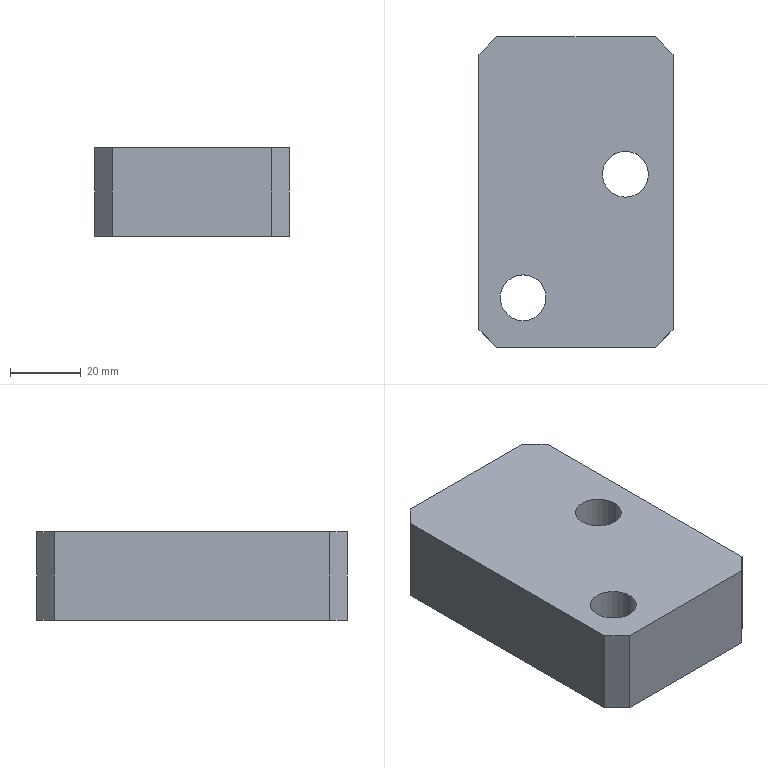Part | STEP file | gslz 2016.10.28-10_id2070_x_t | 1 solid | 16 faces | box 55 x 88 x 25 mm | volume 107688 mm3 | plane 12 | cylinder 4 | commonest cylinder face diameters 13 x2 20 x2
STEP:
#1=CARTESIAN_POINT('',(0.,0.,0.));
#2=DIRECTION('',(0.,0.,1.));
#3=DIRECTION('',(1.,0.,0.));
#4=AXIS2_PLACEMENT_3D('',#1,#2,#3);
#5=CARTESIAN_POINT('',(494.,-313.071,3.));
#6=VERTEX_POINT('',#5);
#7=CARTESIAN_POINT('',(494.,-235.,3.));
#8=VERTEX_POINT('',#7);
#9=CARTESIAN_POINT('',(494.,635.206,3.));
#10=DIRECTION('',(0.,1.,0.));
#11=VECTOR('',#10,1.);
#12=LINE('',#9,#11);
#13=CARTESIAN_POINT('',(494.,627.983,-1.));
#14=DIRECTION('',(-1.,0.,0.));
#15=DIRECTION('',(0.,0.,1.));
#16=AXIS2_PLACEMENT_3D('',#13,#14,#15);
#17=PLANE('',#16);
#18=CARTESIAN_POINT('',(4.,7.223));
#19=DIRECTION('',(0.,1.));
#20=VECTOR('',#19,1.);
#21=LINE('',#18,#20);
#22=(GEOMETRIC_REPRESENTATION_CONTEXT(2)PARAMETRIC_REPRESENTATION_CONTEXT()REPRESENTATION_CONTEXT('',''));
#23=DEFINITIONAL_REPRESENTATION('',(#21),#22);
#24=PCURVE('',#17,#23);
#25=CARTESIAN_POINT('',(-138.966,635.206,3.));
#26=DIRECTION('',(0.,0.,1.));
#27=DIRECTION('',(1.,0.,0.));
#28=AXIS2_PLACEMENT_3D('',#25,#26,#27);
#29=PLANE('',#28);
#30=CARTESIAN_POINT('',(632.966,0.));
#31=DIRECTION('',(0.,1.));
#32=VECTOR('',#31,1.);
#33=LINE('',#30,#32);
#34=(GEOMETRIC_REPRESENTATION_CONTEXT(2)PARAMETRIC_REPRESENTATION_CONTEXT()REPRESENTATION_CONTEXT('',''));
#35=DEFINITIONAL_REPRESENTATION('',(#33),#34);
#36=PCURVE('',#29,#35);
#37=SURFACE_CURVE('',#12,(#24,#36),.PCURVE_S1.);
#38=EDGE_CURVE('',#6,#8,#37,.T.);
#39=ORIENTED_EDGE('',*,*,#38,.T.);
#40=CARTESIAN_POINT('',(494.,-235.,-22.));
#41=VERTEX_POINT('',#40);
#42=CARTESIAN_POINT('',(494.,-235.,-17.));
#43=DIRECTION('',(0.,0.,1.));
#44=VECTOR('',#43,1.);
#45=LINE('',#42,#44);
#46=CARTESIAN_POINT('',(-16.,-862.983));
#47=DIRECTION('',(1.,0.));
#48=VECTOR('',#47,1.);
#49=LINE('',#46,#48);
#50=(GEOMETRIC_REPRESENTATION_CONTEXT(2)PARAMETRIC_REPRESENTATION_CONTEXT()REPRESENTATION_CONTEXT('',''));
#51=DEFINITIONAL_REPRESENTATION('',(#49),#50);
#52=PCURVE('',#17,#51);
#53=CARTESIAN_POINT('',(494.,-235.,-1.));
#54=DIRECTION('',(0.7071,-0.7071,0.));
#55=DIRECTION('',(0.,0.,1.));
#56=AXIS2_PLACEMENT_3D('',#53,#54,#55);
#57=PLANE('',#56);
#58=CARTESIAN_POINT('',(-16.,0.));
#59=DIRECTION('',(1.,0.));
#60=VECTOR('',#59,1.);
#61=LINE('',#58,#60);
#62=(GEOMETRIC_REPRESENTATION_CONTEXT(2)PARAMETRIC_REPRESENTATION_CONTEXT()REPRESENTATION_CONTEXT('',''));
#63=DEFINITIONAL_REPRESENTATION('',(#61),#62);
#64=PCURVE('',#57,#63);
#65=SURFACE_CURVE('',#45,(#52,#64),.PCURVE_S1.);
#66=EDGE_CURVE('',#41,#8,#65,.T.);
#67=ORIENTED_EDGE('',*,*,#66,.F.);
#68=CARTESIAN_POINT('',(494.,-313.071,-22.));
#69=VERTEX_POINT('',#68);
#70=CARTESIAN_POINT('',(494.,635.206,-22.));
#71=DIRECTION('',(0.,1.,0.));
#72=VECTOR('',#71,1.);
#73=LINE('',#70,#72);
#74=CARTESIAN_POINT('',(-21.,7.223));
#75=DIRECTION('',(0.,1.));
#76=VECTOR('',#75,1.);
#77=LINE('',#74,#76);
#78=(GEOMETRIC_REPRESENTATION_CONTEXT(2)PARAMETRIC_REPRESENTATION_CONTEXT()REPRESENTATION_CONTEXT('',''));
#79=DEFINITIONAL_REPRESENTATION('',(#77),#78);
#80=PCURVE('',#17,#79);
#81=CARTESIAN_POINT('',(-138.966,635.206,-22.));
#82=DIRECTION('',(0.,0.,1.));
#83=DIRECTION('',(1.,0.,0.));
#84=AXIS2_PLACEMENT_3D('',#81,#82,#83);
#85=PLANE('',#84);
#86=CARTESIAN_POINT('',(632.966,0.));
#87=DIRECTION('',(0.,1.));
#88=VECTOR('',#87,1.);
#89=LINE('',#86,#88);
#90=(GEOMETRIC_REPRESENTATION_CONTEXT(2)PARAMETRIC_REPRESENTATION_CONTEXT()REPRESENTATION_CONTEXT('',''));
#91=DEFINITIONAL_REPRESENTATION('',(#89),#90);
#92=PCURVE('',#85,#91);
#93=SURFACE_CURVE('',#73,(#80,#92),.PCURVE_S1.);
#94=EDGE_CURVE('',#69,#41,#93,.T.);
#95=ORIENTED_EDGE('',*,*,#94,.F.);
#96=CARTESIAN_POINT('',(494.,-313.071,-1.));
#97=DIRECTION('',(0.,0.,-1.));
#98=VECTOR('',#97,1.);
#99=LINE('',#96,#98);
#100=CARTESIAN_POINT('',(0.,-941.054));
#101=DIRECTION('',(-1.,0.));
#102=VECTOR('',#101,1.);
#103=LINE('',#100,#102);
#104=(GEOMETRIC_REPRESENTATION_CONTEXT(2)PARAMETRIC_REPRESENTATION_CONTEXT()REPRESENTATION_CONTEXT('',''));
#105=DEFINITIONAL_REPRESENTATION('',(#103),#104);
#106=PCURVE('',#17,#105);
#107=CARTESIAN_POINT('',(497.464,-316.536,49.));
#108=DIRECTION('',(0.7071,0.7071,0.));
#109=DIRECTION('',(0.,0.,1.));
#110=AXIS2_PLACEMENT_3D('',#107,#108,#109);
#111=PLANE('',#110);
#112=CARTESIAN_POINT('',(-50.,-4.899));
#113=DIRECTION('',(-1.,0.));
#114=VECTOR('',#113,1.);
#115=LINE('',#112,#114);
#116=(GEOMETRIC_REPRESENTATION_CONTEXT(2)PARAMETRIC_REPRESENTATION_CONTEXT()REPRESENTATION_CONTEXT('',''));
#117=DEFINITIONAL_REPRESENTATION('',(#115),#116);
#118=PCURVE('',#111,#117);
#119=SURFACE_CURVE('',#99,(#106,#118),.PCURVE_S1.);
#120=EDGE_CURVE('',#6,#69,#119,.T.);
#121=ORIENTED_EDGE('',*,*,#120,.F.);
#122=EDGE_LOOP('',(#39,#67,#95,#121));
#123=FACE_BOUND('',#122,.T.);
#124=ADVANCED_FACE('',(#123),#17,.T.);
#125=CARTESIAN_POINT('',(549.,-235.,-22.));
#126=VERTEX_POINT('',#125);
#127=CARTESIAN_POINT('',(549.,-313.071,-22.));
#128=VERTEX_POINT('',#127);
#129=CARTESIAN_POINT('',(549.,635.206,-22.));
#130=DIRECTION('',(0.,-1.,0.));
#131=VECTOR('',#130,1.);
#132=LINE('',#129,#131);
#133=CARTESIAN_POINT('',(549.,627.983,-1.));
#134=DIRECTION('',(1.,0.,0.));
#135=DIRECTION('',(0.,0.,-1.));
#136=AXIS2_PLACEMENT_3D('',#133,#134,#135);
#137=PLANE('',#136);
#138=CARTESIAN_POINT('',(21.,7.223));
#139=DIRECTION('',(0.,-1.));
#140=VECTOR('',#139,1.);
#141=LINE('',#138,#140);
#142=(GEOMETRIC_REPRESENTATION_CONTEXT(2)PARAMETRIC_REPRESENTATION_CONTEXT()REPRESENTATION_CONTEXT('',''));
#143=DEFINITIONAL_REPRESENTATION('',(#141),#142);
#144=PCURVE('',#137,#143);
#145=CARTESIAN_POINT('',(687.966,0.));
#146=DIRECTION('',(0.,-1.));
#147=VECTOR('',#146,1.);
#148=LINE('',#145,#147);
#149=(GEOMETRIC_REPRESENTATION_CONTEXT(2)PARAMETRIC_REPRESENTATION_CONTEXT()REPRESENTATION_CONTEXT('',''));
#150=DEFINITIONAL_REPRESENTATION('',(#148),#149);
#151=PCURVE('',#85,#150);
#152=SURFACE_CURVE('',#132,(#144,#151),.PCURVE_S1.);
#153=EDGE_CURVE('',#126,#128,#152,.T.);
#154=ORIENTED_EDGE('',*,*,#153,.F.);
#155=CARTESIAN_POINT('',(549.,-235.,3.));
#156=VERTEX_POINT('',#155);
#157=CARTESIAN_POINT('',(549.,-235.,3.));
#158=DIRECTION('',(0.,0.,-1.));
#159=VECTOR('',#158,1.);
#160=LINE('',#157,#159);
#161=CARTESIAN_POINT('',(-4.,-862.983));
#162=DIRECTION('',(1.,0.));
#163=VECTOR('',#162,1.);
#164=LINE('',#161,#163);
#165=(GEOMETRIC_REPRESENTATION_CONTEXT(2)PARAMETRIC_REPRESENTATION_CONTEXT()REPRESENTATION_CONTEXT('',''));
#166=DEFINITIONAL_REPRESENTATION('',(#164),#165);
#167=PCURVE('',#137,#166);
#168=CARTESIAN_POINT('',(544.,-230.,4.));
#169=DIRECTION('',(-0.7071,-0.7071,0.));
#170=DIRECTION('',(0.,0.,1.));
#171=AXIS2_PLACEMENT_3D('',#168,#169,#170);
#172=PLANE('',#171);
#173=CARTESIAN_POINT('',(-1.,-7.071));
#174=DIRECTION('',(-1.,0.));
#175=VECTOR('',#174,1.);
#176=LINE('',#173,#175);
#177=(GEOMETRIC_REPRESENTATION_CONTEXT(2)PARAMETRIC_REPRESENTATION_CONTEXT()REPRESENTATION_CONTEXT('',''));
#178=DEFINITIONAL_REPRESENTATION('',(#176),#177);
#179=PCURVE('',#172,#178);
#180=SURFACE_CURVE('',#160,(#167,#179),.PCURVE_S1.);
#181=EDGE_CURVE('',#156,#126,#180,.T.);
#182=ORIENTED_EDGE('',*,*,#181,.F.);
#183=CARTESIAN_POINT('',(549.,-313.071,3.));
#184=VERTEX_POINT('',#183);
#185=CARTESIAN_POINT('',(549.,635.206,3.));
#186=DIRECTION('',(0.,-1.,0.));
#187=VECTOR('',#186,1.);
#188=LINE('',#185,#187);
#189=CARTESIAN_POINT('',(-4.,7.223));
#190=DIRECTION('',(0.,-1.));
#191=VECTOR('',#190,1.);
#192=LINE('',#189,#191);
#193=(GEOMETRIC_REPRESENTATION_CONTEXT(2)PARAMETRIC_REPRESENTATION_CONTEXT()REPRESENTATION_CONTEXT('',''));
#194=DEFINITIONAL_REPRESENTATION('',(#192),#193);
#195=PCURVE('',#137,#194);
#196=CARTESIAN_POINT('',(687.966,0.));
#197=DIRECTION('',(0.,-1.));
#198=VECTOR('',#197,1.);
#199=LINE('',#196,#198);
#200=(GEOMETRIC_REPRESENTATION_CONTEXT(2)PARAMETRIC_REPRESENTATION_CONTEXT()REPRESENTATION_CONTEXT('',''));
#201=DEFINITIONAL_REPRESENTATION('',(#199),#200);
#202=PCURVE('',#29,#201);
#203=SURFACE_CURVE('',#188,(#195,#202),.PCURVE_S1.);
#204=EDGE_CURVE('',#156,#184,#203,.T.);
#205=ORIENTED_EDGE('',*,*,#204,.T.);
#206=CARTESIAN_POINT('',(549.,-313.071,-1.));
#207=DIRECTION('',(0.,0.,1.));
#208=VECTOR('',#207,1.);
#209=LINE('',#206,#208);
#210=CARTESIAN_POINT('',(0.,-941.054));
#211=DIRECTION('',(-1.,0.));
#212=VECTOR('',#211,1.);
#213=LINE('',#210,#212);
#214=(GEOMETRIC_REPRESENTATION_CONTEXT(2)PARAMETRIC_REPRESENTATION_CONTEXT()REPRESENTATION_CONTEXT('',''));
#215=DEFINITIONAL_REPRESENTATION('',(#213),#214);
#216=PCURVE('',#137,#215);
#217=CARTESIAN_POINT('',(547.536,-314.536,-1.));
#218=DIRECTION('',(-0.7071,0.7071,0.));
#219=DIRECTION('',(0.,0.,1.));
#220=AXIS2_PLACEMENT_3D('',#217,#218,#219);
#221=PLANE('',#220);
#222=CARTESIAN_POINT('',(0.,2.071));
#223=DIRECTION('',(1.,0.));
#224=VECTOR('',#223,1.);
#225=LINE('',#222,#224);
#226=(GEOMETRIC_REPRESENTATION_CONTEXT(2)PARAMETRIC_REPRESENTATION_CONTEXT()REPRESENTATION_CONTEXT('',''));
#227=DEFINITIONAL_REPRESENTATION('',(#225),#226);
#228=PCURVE('',#221,#227);
#229=SURFACE_CURVE('',#209,(#216,#228),.PCURVE_S1.);
#230=EDGE_CURVE('',#128,#184,#229,.T.);
#231=ORIENTED_EDGE('',*,*,#230,.F.);
#232=EDGE_LOOP('',(#154,#182,#205,#231));
#233=FACE_BOUND('',#232,.T.);
#234=ADVANCED_FACE('',(#233),#137,.T.);
#235=CARTESIAN_POINT('',(506.5,-314.,-22.));
#236=VERTEX_POINT('',#235);
#237=CARTESIAN_POINT('',(506.5,-294.,-22.));
#238=VERTEX_POINT('',#237);
#239=CARTESIAN_POINT('',(506.5,-304.,-22.));
#240=DIRECTION('',(0.,0.,-1.));
#241=DIRECTION('',(0.,-1.,0.));
#242=AXIS2_PLACEMENT_3D('',#239,#240,#241);
#243=CIRCLE('',#242,10.);
#244=CARTESIAN_POINT('',(645.466,-949.206));
#245=CARTESIAN_POINT('',(628.146,-949.206));
#246=CARTESIAN_POINT('',(636.806,-934.206));
#247=CARTESIAN_POINT('',(645.466,-919.206));
#248=CARTESIAN_POINT('',(654.127,-934.206));
#249=CARTESIAN_POINT('',(662.787,-949.206));
#250=CARTESIAN_POINT('',(645.466,-949.206));
#251=(BOUNDED_CURVE()B_SPLINE_CURVE(2,(#244,#245,#246,#247,#248,#249,#250),.UNSPECIFIED.,.T.,.F.)B_SPLINE_CURVE_WITH_KNOTS((1,2,2,2,2,1),(-2.094,0.,2.094,4.189,6.283,8.378),.UNSPECIFIED.)CURVE()GEOMETRIC_REPRESENTATION_ITEM()RATIONAL_B_SPLINE_CURVE((1.,0.5,1.,0.5,1.,0.5,1.))REPRESENTATION_ITEM(''));
#252=(GEOMETRIC_REPRESENTATION_CONTEXT(2)PARAMETRIC_REPRESENTATION_CONTEXT()REPRESENTATION_CONTEXT('',''));
#253=DEFINITIONAL_REPRESENTATION('',(#251),#252);
#254=PCURVE('',#85,#253);
#255=CARTESIAN_POINT('',(506.5,-304.,3.));
#256=DIRECTION('',(0.,0.,1.));
#257=DIRECTION('',(1.,0.,0.));
#258=AXIS2_PLACEMENT_3D('',#255,#256,#257);
#259=CYLINDRICAL_SURFACE('',#258,10.);
#260=CARTESIAN_POINT('',(4.712,-25.));
#261=DIRECTION('',(-1.,0.));
#262=VECTOR('',#261,1.);
#263=LINE('',#260,#262);
#264=(GEOMETRIC_REPRESENTATION_CONTEXT(2)PARAMETRIC_REPRESENTATION_CONTEXT()REPRESENTATION_CONTEXT('',''));
#265=DEFINITIONAL_REPRESENTATION('',(#263),#264);
#266=PCURVE('',#259,#265);
#267=SURFACE_CURVE('',#243,(#254,#266),.PCURVE_S1.);
#268=EDGE_CURVE('',#236,#238,#267,.T.);
#269=ORIENTED_EDGE('',*,*,#268,.F.);
#270=CARTESIAN_POINT('',(506.5,-304.,-22.));
#271=DIRECTION('',(0.,0.,-1.));
#272=DIRECTION('',(0.,-1.,0.));
#273=AXIS2_PLACEMENT_3D('',#270,#271,#272);
#274=CIRCLE('',#273,10.);
#275=CARTESIAN_POINT('',(645.466,-949.206));
#276=CARTESIAN_POINT('',(628.146,-949.206));
#277=CARTESIAN_POINT('',(636.806,-934.206));
#278=CARTESIAN_POINT('',(645.466,-919.206));
#279=CARTESIAN_POINT('',(654.127,-934.206));
#280=CARTESIAN_POINT('',(662.787,-949.206));
#281=CARTESIAN_POINT('',(645.466,-949.206));
#282=(BOUNDED_CURVE()B_SPLINE_CURVE(2,(#275,#276,#277,#278,#279,#280,#281),.UNSPECIFIED.,.T.,.F.)B_SPLINE_CURVE_WITH_KNOTS((1,2,2,2,2,1),(-2.094,0.,2.094,4.189,6.283,8.378),.UNSPECIFIED.)CURVE()GEOMETRIC_REPRESENTATION_ITEM()RATIONAL_B_SPLINE_CURVE((1.,0.5,1.,0.5,1.,0.5,1.))REPRESENTATION_ITEM(''));
#283=(GEOMETRIC_REPRESENTATION_CONTEXT(2)PARAMETRIC_REPRESENTATION_CONTEXT()REPRESENTATION_CONTEXT('',''));
#284=DEFINITIONAL_REPRESENTATION('',(#282),#283);
#285=PCURVE('',#85,#284);
#286=CARTESIAN_POINT('',(10.996,-25.));
#287=DIRECTION('',(-1.,0.));
#288=VECTOR('',#287,1.);
#289=LINE('',#286,#288);
#290=(GEOMETRIC_REPRESENTATION_CONTEXT(2)PARAMETRIC_REPRESENTATION_CONTEXT()REPRESENTATION_CONTEXT('',''));
#291=DEFINITIONAL_REPRESENTATION('',(#289),#290);
#292=PCURVE('',#259,#291);
#293=SURFACE_CURVE('',#274,(#285,#292),.PCURVE_S1.);
#294=EDGE_CURVE('',#238,#236,#293,.T.);
#295=ORIENTED_EDGE('',*,*,#294,.F.);
#296=EDGE_LOOP('',(#269,#295));
#297=FACE_BOUND('',#296,.T.);
#298=CARTESIAN_POINT('',(535.5,-279.,-22.));
#299=VERTEX_POINT('',#298);
#300=CARTESIAN_POINT('',(535.5,-259.,-22.));
#301=VERTEX_POINT('',#300);
#302=CARTESIAN_POINT('',(535.5,-269.,-22.));
#303=DIRECTION('',(0.,0.,1.));
#304=DIRECTION('',(0.,-1.,0.));
#305=AXIS2_PLACEMENT_3D('',#302,#303,#304);
#306=CIRCLE('',#305,10.);
#307=CARTESIAN_POINT('',(674.466,-904.206));
#308=DIRECTION('',(0.,-1.));
#309=AXIS2_PLACEMENT_2D('',#307,#308);
#310=CIRCLE('',#309,10.);
#311=(GEOMETRIC_REPRESENTATION_CONTEXT(2)PARAMETRIC_REPRESENTATION_CONTEXT()REPRESENTATION_CONTEXT('',''));
#312=DEFINITIONAL_REPRESENTATION('',(#310),#311);
#313=PCURVE('',#85,#312);
#314=CARTESIAN_POINT('',(535.5,-269.,3.));
#315=DIRECTION('',(0.,0.,1.));
#316=DIRECTION('',(1.,0.,0.));
#317=AXIS2_PLACEMENT_3D('',#314,#315,#316);
#318=CYLINDRICAL_SURFACE('',#317,10.);
#319=CARTESIAN_POINT('',(4.712,-25.));
#320=DIRECTION('',(1.,0.));
#321=VECTOR('',#320,1.);
#322=LINE('',#319,#321);
#323=(GEOMETRIC_REPRESENTATION_CONTEXT(2)PARAMETRIC_REPRESENTATION_CONTEXT()REPRESENTATION_CONTEXT('',''));
#324=DEFINITIONAL_REPRESENTATION('',(#322),#323);
#325=PCURVE('',#318,#324);
#326=SURFACE_CURVE('',#306,(#313,#325),.PCURVE_S1.);
#327=EDGE_CURVE('',#299,#301,#326,.T.);
#328=ORIENTED_EDGE('',*,*,#327,.T.);
#329=CARTESIAN_POINT('',(535.5,-269.,-22.));
#330=DIRECTION('',(0.,0.,1.));
#331=DIRECTION('',(0.,-1.,0.));
#332=AXIS2_PLACEMENT_3D('',#329,#330,#331);
#333=CIRCLE('',#332,10.);
#334=CARTESIAN_POINT('',(674.466,-904.206));
#335=DIRECTION('',(0.,-1.));
#336=AXIS2_PLACEMENT_2D('',#334,#335);
#337=CIRCLE('',#336,10.);
#338=(GEOMETRIC_REPRESENTATION_CONTEXT(2)PARAMETRIC_REPRESENTATION_CONTEXT()REPRESENTATION_CONTEXT('',''));
#339=DEFINITIONAL_REPRESENTATION('',(#337),#338);
#340=PCURVE('',#85,#339);
#341=CARTESIAN_POINT('',(-1.571,-25.));
#342=DIRECTION('',(1.,0.));
#343=VECTOR('',#342,1.);
#344=LINE('',#341,#343);
#345=(GEOMETRIC_REPRESENTATION_CONTEXT(2)PARAMETRIC_REPRESENTATION_CONTEXT()REPRESENTATION_CONTEXT('',''));
#346=DEFINITIONAL_REPRESENTATION('',(#344),#345);
#347=PCURVE('',#318,#346);
#348=SURFACE_CURVE('',#333,(#340,#347),.PCURVE_S1.);
#349=EDGE_CURVE('',#301,#299,#348,.T.);
#350=ORIENTED_EDGE('',*,*,#349,.T.);
#351=EDGE_LOOP('',(#328,#350));
#352=FACE_BOUND('',#351,.T.);
#353=CARTESIAN_POINT('',(499.,-230.,-22.));
#354=VERTEX_POINT('',#353);
#355=CARTESIAN_POINT('',(544.,-230.,-22.));
#356=VERTEX_POINT('',#355);
#357=CARTESIAN_POINT('',(-138.966,-230.,-22.));
#358=DIRECTION('',(1.,0.,0.));
#359=VECTOR('',#358,1.);
#360=LINE('',#357,#359);
#361=CARTESIAN_POINT('',(0.,-865.206));
#362=DIRECTION('',(1.,0.));
#363=VECTOR('',#362,1.);
#364=LINE('',#361,#363);
#365=(GEOMETRIC_REPRESENTATION_CONTEXT(2)PARAMETRIC_REPRESENTATION_CONTEXT()REPRESENTATION_CONTEXT('',''));
#366=DEFINITIONAL_REPRESENTATION('',(#364),#365);
#367=PCURVE('',#85,#366);
#368=CARTESIAN_POINT('',(-137.035,-230.,4.));
#369=DIRECTION('',(0.,1.,0.));
#370=DIRECTION('',(-1.,0.,0.));
#371=AXIS2_PLACEMENT_3D('',#368,#369,#370);
#372=PLANE('',#371);
#373=CARTESIAN_POINT('',(1.931,-26.));
#374=DIRECTION('',(-1.,0.));
#375=VECTOR('',#374,1.);
#376=LINE('',#373,#375);
#377=(GEOMETRIC_REPRESENTATION_CONTEXT(2)PARAMETRIC_REPRESENTATION_CONTEXT()REPRESENTATION_CONTEXT('',''));
#378=DEFINITIONAL_REPRESENTATION('',(#376),#377);
#379=PCURVE('',#372,#378);
#380=SURFACE_CURVE('',#360,(#367,#379),.PCURVE_S1.);
#381=EDGE_CURVE('',#354,#356,#380,.T.);
#382=ORIENTED_EDGE('',*,*,#381,.T.);
#383=CARTESIAN_POINT('',(544.,-230.,-22.));
#384=DIRECTION('',(-0.7071,0.7071,0.));
#385=VECTOR('',#384,1.);
#386=LINE('',#383,#385);
#387=CARTESIAN_POINT('',(682.966,-865.206));
#388=DIRECTION('',(-0.7071,0.7071));
#389=VECTOR('',#388,1.);
#390=LINE('',#387,#389);
#391=(GEOMETRIC_REPRESENTATION_CONTEXT(2)PARAMETRIC_REPRESENTATION_CONTEXT()REPRESENTATION_CONTEXT('',''));
#392=DEFINITIONAL_REPRESENTATION('',(#390),#391);
#393=PCURVE('',#85,#392);
#394=CARTESIAN_POINT('',(-26.,0.));
#395=DIRECTION('',(0.,1.));
#396=VECTOR('',#395,1.);
#397=LINE('',#394,#396);
#398=(GEOMETRIC_REPRESENTATION_CONTEXT(2)PARAMETRIC_REPRESENTATION_CONTEXT()REPRESENTATION_CONTEXT('',''));
#399=DEFINITIONAL_REPRESENTATION('',(#397),#398);
#400=PCURVE('',#172,#399);
#401=SURFACE_CURVE('',#386,(#393,#400),.PCURVE_S1.);
#402=EDGE_CURVE('',#126,#356,#401,.T.);
#403=ORIENTED_EDGE('',*,*,#402,.F.);
#404=ORIENTED_EDGE('',*,*,#153,.T.);
#405=CARTESIAN_POINT('',(544.071,-318.,-22.));
#406=VERTEX_POINT('',#405);
#407=CARTESIAN_POINT('',(547.536,-314.536,-22.));
#408=DIRECTION('',(0.7071,0.7071,0.));
#409=VECTOR('',#408,1.);
#410=LINE('',#407,#409);
#411=CARTESIAN_POINT('',(686.502,-949.741));
#412=DIRECTION('',(0.7071,0.7071));
#413=VECTOR('',#412,1.);
#414=LINE('',#411,#413);
#415=(GEOMETRIC_REPRESENTATION_CONTEXT(2)PARAMETRIC_REPRESENTATION_CONTEXT()REPRESENTATION_CONTEXT('',''));
#416=DEFINITIONAL_REPRESENTATION('',(#414),#415);
#417=PCURVE('',#85,#416);
#418=CARTESIAN_POINT('',(-21.,0.));
#419=DIRECTION('',(0.,1.));
#420=VECTOR('',#419,1.);
#421=LINE('',#418,#420);
#422=(GEOMETRIC_REPRESENTATION_CONTEXT(2)PARAMETRIC_REPRESENTATION_CONTEXT()REPRESENTATION_CONTEXT('',''));
#423=DEFINITIONAL_REPRESENTATION('',(#421),#422);
#424=PCURVE('',#221,#423);
#425=SURFACE_CURVE('',#410,(#417,#424),.PCURVE_S1.);
#426=EDGE_CURVE('',#406,#128,#425,.T.);
#427=ORIENTED_EDGE('',*,*,#426,.F.);
#428=CARTESIAN_POINT('',(498.929,-318.,-22.));
#429=VERTEX_POINT('',#428);
#430=CARTESIAN_POINT('',(-138.966,-318.,-22.));
#431=DIRECTION('',(-1.,0.,0.));
#432=VECTOR('',#431,1.);
#433=LINE('',#430,#432);
#434=CARTESIAN_POINT('',(0.,-953.206));
#435=DIRECTION('',(-1.,0.));
#436=VECTOR('',#435,1.);
#437=LINE('',#434,#436);
#438=(GEOMETRIC_REPRESENTATION_CONTEXT(2)PARAMETRIC_REPRESENTATION_CONTEXT()REPRESENTATION_CONTEXT('',''));
#439=DEFINITIONAL_REPRESENTATION('',(#437),#438);
#440=PCURVE('',#85,#439);
#441=CARTESIAN_POINT('',(501.5,-318.,49.));
#442=DIRECTION('',(0.,-1.,0.));
#443=DIRECTION('',(0.,0.,1.));
#444=AXIS2_PLACEMENT_3D('',#441,#442,#443);
#445=PLANE('',#444);
#446=CARTESIAN_POINT('',(-71.,640.466));
#447=DIRECTION('',(0.,1.));
#448=VECTOR('',#447,1.);
#449=LINE('',#446,#448);
#450=(GEOMETRIC_REPRESENTATION_CONTEXT(2)PARAMETRIC_REPRESENTATION_CONTEXT()REPRESENTATION_CONTEXT('',''));
#451=DEFINITIONAL_REPRESENTATION('',(#449),#450);
#452=PCURVE('',#445,#451);
#453=SURFACE_CURVE('',#433,(#440,#452),.PCURVE_S1.);
#454=EDGE_CURVE('',#406,#429,#453,.T.);
#455=ORIENTED_EDGE('',*,*,#454,.T.);
#456=CARTESIAN_POINT('',(497.464,-316.536,-22.));
#457=DIRECTION('',(0.7071,-0.7071,0.));
#458=VECTOR('',#457,1.);
#459=LINE('',#456,#458);
#460=CARTESIAN_POINT('',(636.431,-951.741));
#461=DIRECTION('',(0.7071,-0.7071));
#462=VECTOR('',#461,1.);
#463=LINE('',#460,#462);
#464=(GEOMETRIC_REPRESENTATION_CONTEXT(2)PARAMETRIC_REPRESENTATION_CONTEXT()REPRESENTATION_CONTEXT('',''));
#465=DEFINITIONAL_REPRESENTATION('',(#463),#464);
#466=PCURVE('',#85,#465);
#467=CARTESIAN_POINT('',(-71.,0.));
#468=DIRECTION('',(0.,1.));
#469=VECTOR('',#468,1.);
#470=LINE('',#467,#469);
#471=(GEOMETRIC_REPRESENTATION_CONTEXT(2)PARAMETRIC_REPRESENTATION_CONTEXT()REPRESENTATION_CONTEXT('',''));
#472=DEFINITIONAL_REPRESENTATION('',(#470),#471);
#473=PCURVE('',#111,#472);
#474=SURFACE_CURVE('',#459,(#466,#473),.PCURVE_S1.);
#475=EDGE_CURVE('',#69,#429,#474,.T.);
#476=ORIENTED_EDGE('',*,*,#475,.F.);
#477=ORIENTED_EDGE('',*,*,#94,.T.);
#478=CARTESIAN_POINT('',(494.,-235.,-22.));
#479=DIRECTION('',(-0.7071,-0.7071,0.));
#480=VECTOR('',#479,1.);
#481=LINE('',#478,#480);
#482=CARTESIAN_POINT('',(632.966,-870.206));
#483=DIRECTION('',(-0.7071,-0.7071));
#484=VECTOR('',#483,1.);
#485=LINE('',#482,#484);
#486=(GEOMETRIC_REPRESENTATION_CONTEXT(2)PARAMETRIC_REPRESENTATION_CONTEXT()REPRESENTATION_CONTEXT('',''));
#487=DEFINITIONAL_REPRESENTATION('',(#485),#486);
#488=PCURVE('',#85,#487);
#489=CARTESIAN_POINT('',(-21.,0.));
#490=DIRECTION('',(0.,1.));
#491=VECTOR('',#490,1.);
#492=LINE('',#489,#491);
#493=(GEOMETRIC_REPRESENTATION_CONTEXT(2)PARAMETRIC_REPRESENTATION_CONTEXT()REPRESENTATION_CONTEXT('',''));
#494=DEFINITIONAL_REPRESENTATION('',(#492),#493);
#495=PCURVE('',#57,#494);
#496=SURFACE_CURVE('',#481,(#488,#495),.PCURVE_S1.);
#497=EDGE_CURVE('',#354,#41,#496,.T.);
#498=ORIENTED_EDGE('',*,*,#497,.F.);
#499=EDGE_LOOP('',(#382,#403,#404,#427,#455,#476,#477,#498));
#500=FACE_BOUND('',#499,.T.);
#501=ADVANCED_FACE('',(#297,#352,#500),#85,.F.);
#502=CARTESIAN_POINT('',(535.5,-275.5,3.));
#503=VERTEX_POINT('',#502);
#504=CARTESIAN_POINT('',(535.5,-269.,3.));
#505=DIRECTION('',(0.,0.,-1.));
#506=DIRECTION('',(0.,-1.,0.));
#507=AXIS2_PLACEMENT_3D('',#504,#505,#506);
#508=CIRCLE('',#507,6.5);
#509=CARTESIAN_POINT('',(674.466,-910.706));
#510=CARTESIAN_POINT('',(663.208,-910.706));
#511=CARTESIAN_POINT('',(668.837,-900.956));
#512=CARTESIAN_POINT('',(674.466,-891.206));
#513=CARTESIAN_POINT('',(680.096,-900.956));
#514=CARTESIAN_POINT('',(685.725,-910.706));
#515=CARTESIAN_POINT('',(674.466,-910.706));
#516=(BOUNDED_CURVE()B_SPLINE_CURVE(2,(#509,#510,#511,#512,#513,#514,#515),.UNSPECIFIED.,.T.,.F.)B_SPLINE_CURVE_WITH_KNOTS((1,2,2,2,2,1),(-2.094,0.,2.094,4.189,6.283,8.378),.UNSPECIFIED.)CURVE()GEOMETRIC_REPRESENTATION_ITEM()RATIONAL_B_SPLINE_CURVE((1.,0.5,1.,0.5,1.,0.5,1.))REPRESENTATION_ITEM(''));
#517=(GEOMETRIC_REPRESENTATION_CONTEXT(2)PARAMETRIC_REPRESENTATION_CONTEXT()REPRESENTATION_CONTEXT('',''));
#518=DEFINITIONAL_REPRESENTATION('',(#516),#517);
#519=PCURVE('',#29,#518);
#520=CARTESIAN_POINT('',(535.5,-269.,-84.));
#521=DIRECTION('',(0.,0.,1.));
#522=DIRECTION('',(0.,-1.,0.));
#523=AXIS2_PLACEMENT_3D('',#520,#521,#522);
#524=CYLINDRICAL_SURFACE('',#523,6.5);
#525=CARTESIAN_POINT('',(6.283,87.));
#526=DIRECTION('',(-1.,0.));
#527=VECTOR('',#526,1.);
#528=LINE('',#525,#527);
#529=(GEOMETRIC_REPRESENTATION_CONTEXT(2)PARAMETRIC_REPRESENTATION_CONTEXT()REPRESENTATION_CONTEXT('',''));
#530=DEFINITIONAL_REPRESENTATION('',(#528),#529);
#531=PCURVE('',#524,#530);
#532=SURFACE_CURVE('',#508,(#519,#531),.PCURVE_S1.);
#533=EDGE_CURVE('',#503,#503,#532,.T.);
#534=ORIENTED_EDGE('',*,*,#533,.T.);
#535=EDGE_LOOP('',(#534));
#536=FACE_BOUND('',#535,.T.);
#537=CARTESIAN_POINT('',(506.5,-310.5,3.));
#538=VERTEX_POINT('',#537);
#539=CARTESIAN_POINT('',(506.5,-304.,3.));
#540=DIRECTION('',(0.,0.,-1.));
#541=DIRECTION('',(0.,-1.,0.));
#542=AXIS2_PLACEMENT_3D('',#539,#540,#541);
#543=CIRCLE('',#542,6.5);
#544=CARTESIAN_POINT('',(645.466,-945.706));
#545=CARTESIAN_POINT('',(634.208,-945.706));
#546=CARTESIAN_POINT('',(639.837,-935.956));
#547=CARTESIAN_POINT('',(645.466,-926.206));
#548=CARTESIAN_POINT('',(651.096,-935.956));
#549=CARTESIAN_POINT('',(656.725,-945.706));
#550=CARTESIAN_POINT('',(645.466,-945.706));
#551=(BOUNDED_CURVE()B_SPLINE_CURVE(2,(#544,#545,#546,#547,#548,#549,#550),.UNSPECIFIED.,.T.,.F.)B_SPLINE_CURVE_WITH_KNOTS((1,2,2,2,2,1),(-2.094,0.,2.094,4.189,6.283,8.378),.UNSPECIFIED.)CURVE()GEOMETRIC_REPRESENTATION_ITEM()RATIONAL_B_SPLINE_CURVE((1.,0.5,1.,0.5,1.,0.5,1.))REPRESENTATION_ITEM(''));
#552=(GEOMETRIC_REPRESENTATION_CONTEXT(2)PARAMETRIC_REPRESENTATION_CONTEXT()REPRESENTATION_CONTEXT('',''));
#553=DEFINITIONAL_REPRESENTATION('',(#551),#552);
#554=PCURVE('',#29,#553);
#555=CARTESIAN_POINT('',(506.5,-304.,-84.));
#556=DIRECTION('',(0.,0.,1.));
#557=DIRECTION('',(0.,-1.,0.));
#558=AXIS2_PLACEMENT_3D('',#555,#556,#557);
#559=CYLINDRICAL_SURFACE('',#558,6.5);
#560=CARTESIAN_POINT('',(6.283,87.));
#561=DIRECTION('',(-1.,0.));
#562=VECTOR('',#561,1.);
#563=LINE('',#560,#562);
#564=(GEOMETRIC_REPRESENTATION_CONTEXT(2)PARAMETRIC_REPRESENTATION_CONTEXT()REPRESENTATION_CONTEXT('',''));
#565=DEFINITIONAL_REPRESENTATION('',(#563),#564);
#566=PCURVE('',#559,#565);
#567=SURFACE_CURVE('',#543,(#554,#566),.PCURVE_S1.);
#568=EDGE_CURVE('',#538,#538,#567,.T.);
#569=ORIENTED_EDGE('',*,*,#568,.T.);
#570=EDGE_LOOP('',(#569));
#571=FACE_BOUND('',#570,.T.);
#572=ORIENTED_EDGE('',*,*,#204,.F.);
#573=CARTESIAN_POINT('',(544.,-230.,3.));
#574=VERTEX_POINT('',#573);
#575=CARTESIAN_POINT('',(-227.586,541.586,3.));
#576=DIRECTION('',(0.7071,-0.7071,0.));
#577=VECTOR('',#576,1.);
#578=LINE('',#575,#577);
#579=CARTESIAN_POINT('',(-88.62,-93.62));
#580=DIRECTION('',(0.7071,-0.7071));
#581=VECTOR('',#580,1.);
#582=LINE('',#579,#581);
#583=(GEOMETRIC_REPRESENTATION_CONTEXT(2)PARAMETRIC_REPRESENTATION_CONTEXT()REPRESENTATION_CONTEXT('',''));
#584=DEFINITIONAL_REPRESENTATION('',(#582),#583);
#585=PCURVE('',#29,#584);
#586=CARTESIAN_POINT('',(-1.,1091.187));
#587=DIRECTION('',(0.,-1.));
#588=VECTOR('',#587,1.);
#589=LINE('',#586,#588);
#590=(GEOMETRIC_REPRESENTATION_CONTEXT(2)PARAMETRIC_REPRESENTATION_CONTEXT()REPRESENTATION_CONTEXT('',''));
#591=DEFINITIONAL_REPRESENTATION('',(#589),#590);
#592=PCURVE('',#172,#591);
#593=SURFACE_CURVE('',#578,(#585,#592),.PCURVE_S1.);
#594=EDGE_CURVE('',#574,#156,#593,.T.);
#595=ORIENTED_EDGE('',*,*,#594,.F.);
#596=CARTESIAN_POINT('',(499.,-230.,3.));
#597=VERTEX_POINT('',#596);
#598=CARTESIAN_POINT('',(-138.966,-230.,3.));
#599=DIRECTION('',(1.,0.,0.));
#600=VECTOR('',#599,1.);
#601=LINE('',#598,#600);
#602=CARTESIAN_POINT('',(0.,-865.206));
#603=DIRECTION('',(1.,0.));
#604=VECTOR('',#603,1.);
#605=LINE('',#602,#604);
#606=(GEOMETRIC_REPRESENTATION_CONTEXT(2)PARAMETRIC_REPRESENTATION_CONTEXT()REPRESENTATION_CONTEXT('',''));
#607=DEFINITIONAL_REPRESENTATION('',(#605),#606);
#608=PCURVE('',#29,#607);
#609=CARTESIAN_POINT('',(1.931,-1.));
#610=DIRECTION('',(-1.,0.));
#611=VECTOR('',#610,1.);
#612=LINE('',#609,#611);
#613=(GEOMETRIC_REPRESENTATION_CONTEXT(2)PARAMETRIC_REPRESENTATION_CONTEXT()REPRESENTATION_CONTEXT('',''));
#614=DEFINITIONAL_REPRESENTATION('',(#612),#613);
#615=PCURVE('',#372,#614);
#616=SURFACE_CURVE('',#601,(#608,#615),.PCURVE_S1.);
#617=EDGE_CURVE('',#597,#574,#616,.T.);
#618=ORIENTED_EDGE('',*,*,#617,.F.);
#619=CARTESIAN_POINT('',(630.12,-98.88,3.));
#620=DIRECTION('',(0.7071,0.7071,0.));
#621=VECTOR('',#620,1.);
#622=LINE('',#619,#621);
#623=CARTESIAN_POINT('',(769.086,-734.086));
#624=DIRECTION('',(0.7071,0.7071));
#625=VECTOR('',#624,1.);
#626=LINE('',#623,#625);
#627=(GEOMETRIC_REPRESENTATION_CONTEXT(2)PARAMETRIC_REPRESENTATION_CONTEXT()REPRESENTATION_CONTEXT('',''));
#628=DEFINITIONAL_REPRESENTATION('',(#626),#627);
#629=PCURVE('',#29,#628);
#630=CARTESIAN_POINT('',(4.,-192.502));
#631=DIRECTION('',(0.,-1.));
#632=VECTOR('',#631,1.);
#633=LINE('',#630,#632);
#634=(GEOMETRIC_REPRESENTATION_CONTEXT(2)PARAMETRIC_REPRESENTATION_CONTEXT()REPRESENTATION_CONTEXT('',''));
#635=DEFINITIONAL_REPRESENTATION('',(#633),#634);
#636=PCURVE('',#57,#635);
#637=SURFACE_CURVE('',#622,(#629,#636),.PCURVE_S1.);
#638=EDGE_CURVE('',#8,#597,#637,.T.);
#639=ORIENTED_EDGE('',*,*,#638,.F.);
#640=ORIENTED_EDGE('',*,*,#38,.F.);
#641=CARTESIAN_POINT('',(498.929,-318.,3.));
#642=VERTEX_POINT('',#641);
#643=CARTESIAN_POINT('',(-277.621,458.55,3.));
#644=DIRECTION('',(-0.7071,0.7071,0.));
#645=VECTOR('',#644,1.);
#646=LINE('',#643,#645);
#647=CARTESIAN_POINT('',(-138.655,-176.655));
#648=DIRECTION('',(-0.7071,0.7071));
#649=VECTOR('',#648,1.);
#650=LINE('',#647,#649);
#651=(GEOMETRIC_REPRESENTATION_CONTEXT(2)PARAMETRIC_REPRESENTATION_CONTEXT()REPRESENTATION_CONTEXT('',''));
#652=DEFINITIONAL_REPRESENTATION('',(#650),#651);
#653=PCURVE('',#29,#652);
#654=CARTESIAN_POINT('',(-46.,-1096.137));
#655=DIRECTION('',(0.,-1.));
#656=VECTOR('',#655,1.);
#657=LINE('',#654,#656);
#658=(GEOMETRIC_REPRESENTATION_CONTEXT(2)PARAMETRIC_REPRESENTATION_CONTEXT()REPRESENTATION_CONTEXT('',''));
#659=DEFINITIONAL_REPRESENTATION('',(#657),#658);
#660=PCURVE('',#111,#659);
#661=SURFACE_CURVE('',#646,(#653,#660),.PCURVE_S1.);
#662=EDGE_CURVE('',#642,#6,#661,.T.);
#663=ORIENTED_EDGE('',*,*,#662,.F.);
#664=CARTESIAN_POINT('',(544.071,-318.,3.));
#665=VERTEX_POINT('',#664);
#666=CARTESIAN_POINT('',(-138.966,-318.,3.));
#667=DIRECTION('',(-1.,0.,0.));
#668=VECTOR('',#667,1.);
#669=LINE('',#666,#668);
#670=CARTESIAN_POINT('',(0.,-953.206));
#671=DIRECTION('',(-1.,0.));
#672=VECTOR('',#671,1.);
#673=LINE('',#670,#672);
#674=(GEOMETRIC_REPRESENTATION_CONTEXT(2)PARAMETRIC_REPRESENTATION_CONTEXT()REPRESENTATION_CONTEXT('',''));
#675=DEFINITIONAL_REPRESENTATION('',(#673),#674);
#676=PCURVE('',#29,#675);
#677=CARTESIAN_POINT('',(-46.,640.466));
#678=DIRECTION('',(0.,1.));
#679=VECTOR('',#678,1.);
#680=LINE('',#677,#679);
#681=(GEOMETRIC_REPRESENTATION_CONTEXT(2)PARAMETRIC_REPRESENTATION_CONTEXT()REPRESENTATION_CONTEXT('',''));
#682=DEFINITIONAL_REPRESENTATION('',(#680),#681);
#683=PCURVE('',#445,#682);
#684=SURFACE_CURVE('',#669,(#676,#683),.PCURVE_S1.);
#685=EDGE_CURVE('',#665,#642,#684,.T.);
#686=ORIENTED_EDGE('',*,*,#685,.F.);
#687=CARTESIAN_POINT('',(680.155,-181.916,3.));
#688=DIRECTION('',(-0.7071,-0.7071,0.));
#689=VECTOR('',#688,1.);
#690=LINE('',#687,#689);
#691=CARTESIAN_POINT('',(819.121,-817.121));
#692=DIRECTION('',(-0.7071,-0.7071));
#693=VECTOR('',#692,1.);
#694=LINE('',#691,#693);
#695=(GEOMETRIC_REPRESENTATION_CONTEXT(2)PARAMETRIC_REPRESENTATION_CONTEXT()REPRESENTATION_CONTEXT('',''));
#696=DEFINITIONAL_REPRESENTATION('',(#694),#695);
#697=PCURVE('',#29,#696);
#698=CARTESIAN_POINT('',(4.,187.552));
#699=DIRECTION('',(0.,-1.));
#700=VECTOR('',#699,1.);
#701=LINE('',#698,#700);
#702=(GEOMETRIC_REPRESENTATION_CONTEXT(2)PARAMETRIC_REPRESENTATION_CONTEXT()REPRESENTATION_CONTEXT('',''));
#703=DEFINITIONAL_REPRESENTATION('',(#701),#702);
#704=PCURVE('',#221,#703);
#705=SURFACE_CURVE('',#690,(#697,#704),.PCURVE_S1.);
#706=EDGE_CURVE('',#184,#665,#705,.T.);
#707=ORIENTED_EDGE('',*,*,#706,.F.);
#708=EDGE_LOOP('',(#572,#595,#618,#639,#640,#663,#686,#707));
#709=FACE_BOUND('',#708,.T.);
#710=ADVANCED_FACE('',(#536,#571,#709),#29,.T.);
#711=CARTESIAN_POINT('',(535.5,-259.,-7.));
#712=VERTEX_POINT('',#711);
#713=CARTESIAN_POINT('',(535.5,-269.,-7.));
#714=DIRECTION('',(0.,0.,1.));
#715=DIRECTION('',(0.,1.,0.));
#716=AXIS2_PLACEMENT_3D('',#713,#714,#715);
#717=CIRCLE('',#716,10.);
#718=CARTESIAN_POINT('',(535.5,-269.,-7.));
#719=DIRECTION('',(0.,0.,-1.));
#720=DIRECTION('',(0.,1.,0.));
#721=AXIS2_PLACEMENT_3D('',#718,#719,#720);
#722=PLANE('',#721);
#723=CARTESIAN_POINT('',(10.,0.));
#724=CARTESIAN_POINT('',(10.,-17.321));
#725=CARTESIAN_POINT('',(-5.,-8.66));
#726=CARTESIAN_POINT('',(-20.,0.));
#727=CARTESIAN_POINT('',(-5.,8.66));
#728=CARTESIAN_POINT('',(10.,17.321));
#729=CARTESIAN_POINT('',(10.,0.));
#730=(BOUNDED_CURVE()B_SPLINE_CURVE(2,(#723,#724,#725,#726,#727,#728,#729),.UNSPECIFIED.,.T.,.F.)B_SPLINE_CURVE_WITH_KNOTS((1,2,2,2,2,1),(-2.094,0.,2.094,4.189,6.283,8.378),.UNSPECIFIED.)CURVE()GEOMETRIC_REPRESENTATION_ITEM()RATIONAL_B_SPLINE_CURVE((1.,0.5,1.,0.5,1.,0.5,1.))REPRESENTATION_ITEM(''));
#731=(GEOMETRIC_REPRESENTATION_CONTEXT(2)PARAMETRIC_REPRESENTATION_CONTEXT()REPRESENTATION_CONTEXT('',''));
#732=DEFINITIONAL_REPRESENTATION('',(#730),#731);
#733=PCURVE('',#722,#732);
#734=CARTESIAN_POINT('',(1.571,-10.));
#735=DIRECTION('',(1.,0.));
#736=VECTOR('',#735,1.);
#737=LINE('',#734,#736);
#738=(GEOMETRIC_REPRESENTATION_CONTEXT(2)PARAMETRIC_REPRESENTATION_CONTEXT()REPRESENTATION_CONTEXT('',''));
#739=DEFINITIONAL_REPRESENTATION('',(#737),#738);
#740=PCURVE('',#318,#739);
#741=SURFACE_CURVE('',#717,(#733,#740),.PCURVE_S1.);
#742=EDGE_CURVE('',#712,#712,#741,.T.);
#743=ORIENTED_EDGE('',*,*,#742,.F.);
#744=EDGE_LOOP('',(#743));
#745=FACE_BOUND('',#744,.T.);
#746=CARTESIAN_POINT('',(535.5,-262.5,-7.));
#747=VERTEX_POINT('',#746);
#748=CARTESIAN_POINT('',(535.5,-275.5,-7.));
#749=VERTEX_POINT('',#748);
#750=CARTESIAN_POINT('',(535.5,-269.,-7.));
#751=DIRECTION('',(0.,0.,-1.));
#752=DIRECTION('',(0.,1.,0.));
#753=AXIS2_PLACEMENT_3D('',#750,#751,#752);
#754=CIRCLE('',#753,6.5);
#755=CARTESIAN_POINT('',(0.,0.));
#756=DIRECTION('',(1.,0.));
#757=AXIS2_PLACEMENT_2D('',#755,#756);
#758=CIRCLE('',#757,6.5);
#759=(GEOMETRIC_REPRESENTATION_CONTEXT(2)PARAMETRIC_REPRESENTATION_CONTEXT()REPRESENTATION_CONTEXT('',''));
#760=DEFINITIONAL_REPRESENTATION('',(#758),#759);
#761=PCURVE('',#722,#760);
#762=CARTESIAN_POINT('',(3.142,77.));
#763=DIRECTION('',(-1.,0.));
#764=VECTOR('',#763,1.);
#765=LINE('',#762,#764);
#766=(GEOMETRIC_REPRESENTATION_CONTEXT(2)PARAMETRIC_REPRESENTATION_CONTEXT()REPRESENTATION_CONTEXT('',''));
#767=DEFINITIONAL_REPRESENTATION('',(#765),#766);
#768=PCURVE('',#524,#767);
#769=SURFACE_CURVE('',#754,(#761,#768),.PCURVE_S1.);
#770=EDGE_CURVE('',#747,#749,#769,.T.);
#771=ORIENTED_EDGE('',*,*,#770,.F.);
#772=CARTESIAN_POINT('',(535.5,-269.,-7.));
#773=DIRECTION('',(0.,0.,-1.));
#774=DIRECTION('',(0.,1.,0.));
#775=AXIS2_PLACEMENT_3D('',#772,#773,#774);
#776=CIRCLE('',#775,6.5);
#777=CARTESIAN_POINT('',(0.,0.));
#778=DIRECTION('',(1.,0.));
#779=AXIS2_PLACEMENT_2D('',#777,#778);
#780=CIRCLE('',#779,6.5);
#781=(GEOMETRIC_REPRESENTATION_CONTEXT(2)PARAMETRIC_REPRESENTATION_CONTEXT()REPRESENTATION_CONTEXT('',''));
#782=DEFINITIONAL_REPRESENTATION('',(#780),#781);
#783=PCURVE('',#722,#782);
#784=CARTESIAN_POINT('',(9.425,77.));
#785=DIRECTION('',(-1.,0.));
#786=VECTOR('',#785,1.);
#787=LINE('',#784,#786);
#788=(GEOMETRIC_REPRESENTATION_CONTEXT(2)PARAMETRIC_REPRESENTATION_CONTEXT()REPRESENTATION_CONTEXT('',''));
#789=DEFINITIONAL_REPRESENTATION('',(#787),#788);
#790=PCURVE('',#524,#789);
#791=SURFACE_CURVE('',#776,(#783,#790),.PCURVE_S1.);
#792=EDGE_CURVE('',#749,#747,#791,.T.);
#793=ORIENTED_EDGE('',*,*,#792,.F.);
#794=EDGE_LOOP('',(#771,#793));
#795=FACE_BOUND('',#794,.T.);
#796=ADVANCED_FACE('',(#745,#795),#722,.T.);
#797=ORIENTED_EDGE('',*,*,#742,.F.);
#798=CARTESIAN_POINT('',(535.5,-259.,-22.));
#799=CARTESIAN_POINT('',(535.5,-259.,-7.));
#800=B_SPLINE_CURVE_WITH_KNOTS('',1,(#798,#799),.UNSPECIFIED.,.F.,.F.,(2,2),(-25.,-10.),.PIECEWISE_BEZIER_KNOTS.);
#801=CARTESIAN_POINT('',(1.571,0.));
#802=DIRECTION('',(0.,1.));
#803=VECTOR('',#802,1.);
#804=LINE('',#801,#803);
#805=(GEOMETRIC_REPRESENTATION_CONTEXT(2)PARAMETRIC_REPRESENTATION_CONTEXT()REPRESENTATION_CONTEXT('',''));
#806=DEFINITIONAL_REPRESENTATION('',(#804),#805);
#807=PCURVE('',#318,#806);
#808=CARTESIAN_POINT('',(7.854,0.));
#809=DIRECTION('',(0.,1.));
#810=VECTOR('',#809,1.);
#811=LINE('',#808,#810);
#812=(GEOMETRIC_REPRESENTATION_CONTEXT(2)PARAMETRIC_REPRESENTATION_CONTEXT()REPRESENTATION_CONTEXT('',''));
#813=DEFINITIONAL_REPRESENTATION('',(#811),#812);
#814=PCURVE('',#318,#813);
#815=SEAM_CURVE('',#800,(#807,#814),.PCURVE_S1.);
#816=EDGE_CURVE('',#301,#712,#815,.T.);
#817=ORIENTED_EDGE('',*,*,#816,.F.);
#818=ORIENTED_EDGE('',*,*,#349,.T.);
#819=ORIENTED_EDGE('',*,*,#327,.T.);
#820=ORIENTED_EDGE('',*,*,#816,.T.);
#821=EDGE_LOOP('',(#797,#817,#818,#819,#820));
#822=FACE_BOUND('',#821,.F.);
#823=ADVANCED_FACE('',(#822),#318,.F.);
#824=ORIENTED_EDGE('',*,*,#533,.T.);
#825=CARTESIAN_POINT('',(535.5,-275.5,-7.));
#826=CARTESIAN_POINT('',(535.5,-275.5,3.));
#827=B_SPLINE_CURVE_WITH_KNOTS('',1,(#825,#826),.UNSPECIFIED.,.F.,.F.,(2,2),(77.,87.),.PIECEWISE_BEZIER_KNOTS.);
#828=CARTESIAN_POINT('',(0.,0.));
#829=DIRECTION('',(0.,1.));
#830=VECTOR('',#829,1.);
#831=LINE('',#828,#830);
#832=(GEOMETRIC_REPRESENTATION_CONTEXT(2)PARAMETRIC_REPRESENTATION_CONTEXT()REPRESENTATION_CONTEXT('',''));
#833=DEFINITIONAL_REPRESENTATION('',(#831),#832);
#834=PCURVE('',#524,#833);
#835=CARTESIAN_POINT('',(6.283,0.));
#836=DIRECTION('',(0.,1.));
#837=VECTOR('',#836,1.);
#838=LINE('',#835,#837);
#839=(GEOMETRIC_REPRESENTATION_CONTEXT(2)PARAMETRIC_REPRESENTATION_CONTEXT()REPRESENTATION_CONTEXT('',''));
#840=DEFINITIONAL_REPRESENTATION('',(#838),#839);
#841=PCURVE('',#524,#840);
#842=SEAM_CURVE('',#827,(#834,#841),.PCURVE_S1.);
#843=EDGE_CURVE('',#749,#503,#842,.T.);
#844=ORIENTED_EDGE('',*,*,#843,.F.);
#845=ORIENTED_EDGE('',*,*,#770,.F.);
#846=ORIENTED_EDGE('',*,*,#792,.F.);
#847=ORIENTED_EDGE('',*,*,#843,.T.);
#848=EDGE_LOOP('',(#824,#844,#845,#846,#847));
#849=FACE_BOUND('',#848,.F.);
#850=ADVANCED_FACE('',(#849),#524,.F.);
#851=CARTESIAN_POINT('',(506.5,-294.,-7.));
#852=VERTEX_POINT('',#851);
#853=CARTESIAN_POINT('',(506.5,-304.,-7.));
#854=DIRECTION('',(0.,0.,1.));
#855=DIRECTION('',(0.,1.,0.));
#856=AXIS2_PLACEMENT_3D('',#853,#854,#855);
#857=CIRCLE('',#856,10.);
#858=CARTESIAN_POINT('',(506.5,-304.,-7.));
#859=DIRECTION('',(0.,0.,-1.));
#860=DIRECTION('',(0.,1.,0.));
#861=AXIS2_PLACEMENT_3D('',#858,#859,#860);
#862=PLANE('',#861);
#863=CARTESIAN_POINT('',(10.,0.));
#864=CARTESIAN_POINT('',(10.,-17.321));
#865=CARTESIAN_POINT('',(-5.,-8.66));
#866=CARTESIAN_POINT('',(-20.,0.));
#867=CARTESIAN_POINT('',(-5.,8.66));
#868=CARTESIAN_POINT('',(10.,17.321));
#869=CARTESIAN_POINT('',(10.,0.));
#870=(BOUNDED_CURVE()B_SPLINE_CURVE(2,(#863,#864,#865,#866,#867,#868,#869),.UNSPECIFIED.,.T.,.F.)B_SPLINE_CURVE_WITH_KNOTS((1,2,2,2,2,1),(-2.094,0.,2.094,4.189,6.283,8.378),.UNSPECIFIED.)CURVE()GEOMETRIC_REPRESENTATION_ITEM()RATIONAL_B_SPLINE_CURVE((1.,0.5,1.,0.5,1.,0.5,1.))REPRESENTATION_ITEM(''));
#871=(GEOMETRIC_REPRESENTATION_CONTEXT(2)PARAMETRIC_REPRESENTATION_CONTEXT()REPRESENTATION_CONTEXT('',''));
#872=DEFINITIONAL_REPRESENTATION('',(#870),#871);
#873=PCURVE('',#862,#872);
#874=CARTESIAN_POINT('',(1.571,-10.));
#875=DIRECTION('',(1.,0.));
#876=VECTOR('',#875,1.);
#877=LINE('',#874,#876);
#878=(GEOMETRIC_REPRESENTATION_CONTEXT(2)PARAMETRIC_REPRESENTATION_CONTEXT()REPRESENTATION_CONTEXT('',''));
#879=DEFINITIONAL_REPRESENTATION('',(#877),#878);
#880=PCURVE('',#259,#879);
#881=SURFACE_CURVE('',#857,(#873,#880),.PCURVE_S1.);
#882=EDGE_CURVE('',#852,#852,#881,.T.);
#883=ORIENTED_EDGE('',*,*,#882,.F.);
#884=EDGE_LOOP('',(#883));
#885=FACE_BOUND('',#884,.T.);
#886=CARTESIAN_POINT('',(506.5,-297.5,-7.));
#887=VERTEX_POINT('',#886);
#888=CARTESIAN_POINT('',(506.5,-310.5,-7.));
#889=VERTEX_POINT('',#888);
#890=CARTESIAN_POINT('',(506.5,-304.,-7.));
#891=DIRECTION('',(0.,0.,-1.));
#892=DIRECTION('',(0.,1.,0.));
#893=AXIS2_PLACEMENT_3D('',#890,#891,#892);
#894=CIRCLE('',#893,6.5);
#895=CARTESIAN_POINT('',(0.,0.));
#896=DIRECTION('',(1.,0.));
#897=AXIS2_PLACEMENT_2D('',#895,#896);
#898=CIRCLE('',#897,6.5);
#899=(GEOMETRIC_REPRESENTATION_CONTEXT(2)PARAMETRIC_REPRESENTATION_CONTEXT()REPRESENTATION_CONTEXT('',''));
#900=DEFINITIONAL_REPRESENTATION('',(#898),#899);
#901=PCURVE('',#862,#900);
#902=CARTESIAN_POINT('',(3.142,77.));
#903=DIRECTION('',(-1.,0.));
#904=VECTOR('',#903,1.);
#905=LINE('',#902,#904);
#906=(GEOMETRIC_REPRESENTATION_CONTEXT(2)PARAMETRIC_REPRESENTATION_CONTEXT()REPRESENTATION_CONTEXT('',''));
#907=DEFINITIONAL_REPRESENTATION('',(#905),#906);
#908=PCURVE('',#559,#907);
#909=SURFACE_CURVE('',#894,(#901,#908),.PCURVE_S1.);
#910=EDGE_CURVE('',#887,#889,#909,.T.);
#911=ORIENTED_EDGE('',*,*,#910,.F.);
#912=CARTESIAN_POINT('',(506.5,-304.,-7.));
#913=DIRECTION('',(0.,0.,-1.));
#914=DIRECTION('',(0.,1.,0.));
#915=AXIS2_PLACEMENT_3D('',#912,#913,#914);
#916=CIRCLE('',#915,6.5);
#917=CARTESIAN_POINT('',(0.,0.));
#918=DIRECTION('',(1.,0.));
#919=AXIS2_PLACEMENT_2D('',#917,#918);
#920=CIRCLE('',#919,6.5);
#921=(GEOMETRIC_REPRESENTATION_CONTEXT(2)PARAMETRIC_REPRESENTATION_CONTEXT()REPRESENTATION_CONTEXT('',''));
#922=DEFINITIONAL_REPRESENTATION('',(#920),#921);
#923=PCURVE('',#862,#922);
#924=CARTESIAN_POINT('',(9.425,77.));
#925=DIRECTION('',(-1.,0.));
#926=VECTOR('',#925,1.);
#927=LINE('',#924,#926);
#928=(GEOMETRIC_REPRESENTATION_CONTEXT(2)PARAMETRIC_REPRESENTATION_CONTEXT()REPRESENTATION_CONTEXT('',''));
#929=DEFINITIONAL_REPRESENTATION('',(#927),#928);
#930=PCURVE('',#559,#929);
#931=SURFACE_CURVE('',#916,(#923,#930),.PCURVE_S1.);
#932=EDGE_CURVE('',#889,#887,#931,.T.);
#933=ORIENTED_EDGE('',*,*,#932,.F.);
#934=EDGE_LOOP('',(#911,#933));
#935=FACE_BOUND('',#934,.T.);
#936=ADVANCED_FACE('',(#885,#935),#862,.T.);
#937=ORIENTED_EDGE('',*,*,#568,.T.);
#938=CARTESIAN_POINT('',(506.5,-310.5,-7.));
#939=CARTESIAN_POINT('',(506.5,-310.5,3.));
#940=B_SPLINE_CURVE_WITH_KNOTS('',1,(#938,#939),.UNSPECIFIED.,.F.,.F.,(2,2),(77.,87.),.PIECEWISE_BEZIER_KNOTS.);
#941=CARTESIAN_POINT('',(0.,0.));
#942=DIRECTION('',(0.,1.));
#943=VECTOR('',#942,1.);
#944=LINE('',#941,#943);
#945=(GEOMETRIC_REPRESENTATION_CONTEXT(2)PARAMETRIC_REPRESENTATION_CONTEXT()REPRESENTATION_CONTEXT('',''));
#946=DEFINITIONAL_REPRESENTATION('',(#944),#945);
#947=PCURVE('',#559,#946);
#948=CARTESIAN_POINT('',(6.283,0.));
#949=DIRECTION('',(0.,1.));
#950=VECTOR('',#949,1.);
#951=LINE('',#948,#950);
#952=(GEOMETRIC_REPRESENTATION_CONTEXT(2)PARAMETRIC_REPRESENTATION_CONTEXT()REPRESENTATION_CONTEXT('',''));
#953=DEFINITIONAL_REPRESENTATION('',(#951),#952);
#954=PCURVE('',#559,#953);
#955=SEAM_CURVE('',#940,(#947,#954),.PCURVE_S1.);
#956=EDGE_CURVE('',#889,#538,#955,.T.);
#957=ORIENTED_EDGE('',*,*,#956,.F.);
#958=ORIENTED_EDGE('',*,*,#910,.F.);
#959=ORIENTED_EDGE('',*,*,#932,.F.);
#960=ORIENTED_EDGE('',*,*,#956,.T.);
#961=EDGE_LOOP('',(#937,#957,#958,#959,#960));
#962=FACE_BOUND('',#961,.F.);
#963=ADVANCED_FACE('',(#962),#559,.F.);
#964=ORIENTED_EDGE('',*,*,#882,.F.);
#965=CARTESIAN_POINT('',(506.5,-294.,-22.));
#966=CARTESIAN_POINT('',(506.5,-294.,-7.));
#967=B_SPLINE_CURVE_WITH_KNOTS('',1,(#965,#966),.UNSPECIFIED.,.F.,.F.,(2,2),(-25.,-10.),.PIECEWISE_BEZIER_KNOTS.);
#968=CARTESIAN_POINT('',(1.571,0.));
#969=DIRECTION('',(0.,1.));
#970=VECTOR('',#969,1.);
#971=LINE('',#968,#970);
#972=(GEOMETRIC_REPRESENTATION_CONTEXT(2)PARAMETRIC_REPRESENTATION_CONTEXT()REPRESENTATION_CONTEXT('',''));
#973=DEFINITIONAL_REPRESENTATION('',(#971),#972);
#974=PCURVE('',#259,#973);
#975=CARTESIAN_POINT('',(7.854,0.));
#976=DIRECTION('',(0.,1.));
#977=VECTOR('',#976,1.);
#978=LINE('',#975,#977);
#979=(GEOMETRIC_REPRESENTATION_CONTEXT(2)PARAMETRIC_REPRESENTATION_CONTEXT()REPRESENTATION_CONTEXT('',''));
#980=DEFINITIONAL_REPRESENTATION('',(#978),#979);
#981=PCURVE('',#259,#980);
#982=SEAM_CURVE('',#967,(#974,#981),.PCURVE_S1.);
#983=EDGE_CURVE('',#238,#852,#982,.T.);
#984=ORIENTED_EDGE('',*,*,#983,.F.);
#985=ORIENTED_EDGE('',*,*,#268,.F.);
#986=ORIENTED_EDGE('',*,*,#294,.F.);
#987=ORIENTED_EDGE('',*,*,#983,.T.);
#988=EDGE_LOOP('',(#964,#984,#985,#986,#987));
#989=FACE_BOUND('',#988,.F.);
#990=ADVANCED_FACE('',(#989),#259,.F.);
#991=ORIENTED_EDGE('',*,*,#685,.T.);
#992=CARTESIAN_POINT('',(498.929,-318.,49.));
#993=DIRECTION('',(0.,0.,1.));
#994=VECTOR('',#993,1.);
#995=LINE('',#992,#994);
#996=CARTESIAN_POINT('',(0.,2.571));
#997=DIRECTION('',(1.,0.));
#998=VECTOR('',#997,1.);
#999=LINE('',#996,#998);
#1000=(GEOMETRIC_REPRESENTATION_CONTEXT(2)PARAMETRIC_REPRESENTATION_CONTEXT()REPRESENTATION_CONTEXT('',''));
#1001=DEFINITIONAL_REPRESENTATION('',(#999),#1000);
#1002=PCURVE('',#445,#1001);
#1003=CARTESIAN_POINT('',(0.,2.071));
#1004=DIRECTION('',(1.,0.));
#1005=VECTOR('',#1004,1.);
#1006=LINE('',#1003,#1005);
#1007=(GEOMETRIC_REPRESENTATION_CONTEXT(2)PARAMETRIC_REPRESENTATION_CONTEXT()REPRESENTATION_CONTEXT('',''));
#1008=DEFINITIONAL_REPRESENTATION('',(#1006),#1007);
#1009=PCURVE('',#111,#1008);
#1010=SURFACE_CURVE('',#995,(#1002,#1009),.PCURVE_S1.);
#1011=EDGE_CURVE('',#429,#642,#1010,.T.);
#1012=ORIENTED_EDGE('',*,*,#1011,.F.);
#1013=ORIENTED_EDGE('',*,*,#454,.F.);
#1014=CARTESIAN_POINT('',(544.071,-318.,49.));
#1015=DIRECTION('',(0.,0.,-1.));
#1016=VECTOR('',#1015,1.);
#1017=LINE('',#1014,#1016);
#1018=CARTESIAN_POINT('',(0.,-42.571));
#1019=DIRECTION('',(-1.,0.));
#1020=VECTOR('',#1019,1.);
#1021=LINE('',#1018,#1020);
#1022=(GEOMETRIC_REPRESENTATION_CONTEXT(2)PARAMETRIC_REPRESENTATION_CONTEXT()REPRESENTATION_CONTEXT('',''));
#1023=DEFINITIONAL_REPRESENTATION('',(#1021),#1022);
#1024=PCURVE('',#445,#1023);
#1025=CARTESIAN_POINT('',(50.,-4.899));
#1026=DIRECTION('',(-1.,0.));
#1027=VECTOR('',#1026,1.);
#1028=LINE('',#1025,#1027);
#1029=(GEOMETRIC_REPRESENTATION_CONTEXT(2)PARAMETRIC_REPRESENTATION_CONTEXT()REPRESENTATION_CONTEXT('',''));
#1030=DEFINITIONAL_REPRESENTATION('',(#1028),#1029);
#1031=PCURVE('',#221,#1030);
#1032=SURFACE_CURVE('',#1017,(#1024,#1031),.PCURVE_S1.);
#1033=EDGE_CURVE('',#665,#406,#1032,.T.);
#1034=ORIENTED_EDGE('',*,*,#1033,.F.);
#1035=EDGE_LOOP('',(#991,#1012,#1013,#1034));
#1036=FACE_BOUND('',#1035,.T.);
#1037=ADVANCED_FACE('',(#1036),#445,.T.);
#1038=ORIENTED_EDGE('',*,*,#617,.T.);
#1039=CARTESIAN_POINT('',(544.,-230.,-17.));
#1040=DIRECTION('',(0.,0.,1.));
#1041=VECTOR('',#1040,1.);
#1042=LINE('',#1039,#1041);
#1043=CARTESIAN_POINT('',(-681.035,-21.));
#1044=DIRECTION('',(0.,1.));
#1045=VECTOR('',#1044,1.);
#1046=LINE('',#1043,#1045);
#1047=(GEOMETRIC_REPRESENTATION_CONTEXT(2)PARAMETRIC_REPRESENTATION_CONTEXT()REPRESENTATION_CONTEXT('',''));
#1048=DEFINITIONAL_REPRESENTATION('',(#1046),#1047);
#1049=PCURVE('',#372,#1048);
#1050=CARTESIAN_POINT('',(-21.,0.));
#1051=DIRECTION('',(1.,0.));
#1052=VECTOR('',#1051,1.);
#1053=LINE('',#1050,#1052);
#1054=(GEOMETRIC_REPRESENTATION_CONTEXT(2)PARAMETRIC_REPRESENTATION_CONTEXT()REPRESENTATION_CONTEXT('',''));
#1055=DEFINITIONAL_REPRESENTATION('',(#1053),#1054);
#1056=PCURVE('',#172,#1055);
#1057=SURFACE_CURVE('',#1042,(#1049,#1056),.PCURVE_S1.);
#1058=EDGE_CURVE('',#356,#574,#1057,.T.);
#1059=ORIENTED_EDGE('',*,*,#1058,.F.);
#1060=ORIENTED_EDGE('',*,*,#381,.F.);
#1061=CARTESIAN_POINT('',(499.,-230.,3.));
#1062=DIRECTION('',(0.,0.,-1.));
#1063=VECTOR('',#1062,1.);
#1064=LINE('',#1061,#1063);
#1065=CARTESIAN_POINT('',(-636.035,-1.));
#1066=DIRECTION('',(0.,-1.));
#1067=VECTOR('',#1066,1.);
#1068=LINE('',#1065,#1067);
#1069=(GEOMETRIC_REPRESENTATION_CONTEXT(2)PARAMETRIC_REPRESENTATION_CONTEXT()REPRESENTATION_CONTEXT('',''));
#1070=DEFINITIONAL_REPRESENTATION('',(#1068),#1069);
#1071=PCURVE('',#372,#1070);
#1072=CARTESIAN_POINT('',(4.,-7.071));
#1073=DIRECTION('',(-1.,0.));
#1074=VECTOR('',#1073,1.);
#1075=LINE('',#1072,#1074);
#1076=(GEOMETRIC_REPRESENTATION_CONTEXT(2)PARAMETRIC_REPRESENTATION_CONTEXT()REPRESENTATION_CONTEXT('',''));
#1077=DEFINITIONAL_REPRESENTATION('',(#1075),#1076);
#1078=PCURVE('',#57,#1077);
#1079=SURFACE_CURVE('',#1064,(#1071,#1078),.PCURVE_S1.);
#1080=EDGE_CURVE('',#597,#354,#1079,.T.);
#1081=ORIENTED_EDGE('',*,*,#1080,.F.);
#1082=EDGE_LOOP('',(#1038,#1059,#1060,#1081));
#1083=FACE_BOUND('',#1082,.T.);
#1084=ADVANCED_FACE('',(#1083),#372,.T.);
#1085=ORIENTED_EDGE('',*,*,#662,.T.);
#1086=ORIENTED_EDGE('',*,*,#120,.T.);
#1087=ORIENTED_EDGE('',*,*,#475,.T.);
#1088=ORIENTED_EDGE('',*,*,#1011,.T.);
#1089=EDGE_LOOP('',(#1085,#1086,#1087,#1088));
#1090=FACE_BOUND('',#1089,.T.);
#1091=ADVANCED_FACE('',(#1090),#111,.F.);
#1092=ORIENTED_EDGE('',*,*,#706,.T.);
#1093=ORIENTED_EDGE('',*,*,#1033,.T.);
#1094=ORIENTED_EDGE('',*,*,#426,.T.);
#1095=ORIENTED_EDGE('',*,*,#230,.T.);
#1096=EDGE_LOOP('',(#1092,#1093,#1094,#1095));
#1097=FACE_BOUND('',#1096,.T.);
#1098=ADVANCED_FACE('',(#1097),#221,.F.);
#1099=ORIENTED_EDGE('',*,*,#594,.T.);
#1100=ORIENTED_EDGE('',*,*,#181,.T.);
#1101=ORIENTED_EDGE('',*,*,#402,.T.);
#1102=ORIENTED_EDGE('',*,*,#1058,.T.);
#1103=EDGE_LOOP('',(#1099,#1100,#1101,#1102));
#1104=FACE_BOUND('',#1103,.T.);
#1105=ADVANCED_FACE('',(#1104),#172,.F.);
#1106=ORIENTED_EDGE('',*,*,#638,.T.);
#1107=ORIENTED_EDGE('',*,*,#1080,.T.);
#1108=ORIENTED_EDGE('',*,*,#497,.T.);
#1109=ORIENTED_EDGE('',*,*,#66,.T.);
#1110=EDGE_LOOP('',(#1106,#1107,#1108,#1109));
#1111=FACE_BOUND('',#1110,.T.);
#1112=ADVANCED_FACE('',(#1111),#57,.F.);
#1113=CLOSED_SHELL('',(#124,#234,#501,#710,#796,#823,#850,#936,#963,#990,#1037,#1084,#1091,#1098,#1105,#1112));
#1114=MANIFOLD_SOLID_BREP('',#1113);
#1115=(LENGTH_UNIT()NAMED_UNIT(*)SI_UNIT(.MILLI.,.METRE.));
#1116=UNCERTAINTY_MEASURE_WITH_UNIT(LENGTH_MEASURE(0.000002),#1115,'','');
#1117=(NAMED_UNIT(*)PLANE_ANGLE_UNIT()SI_UNIT($,.RADIAN.));
#1118=(NAMED_UNIT(*)SI_UNIT($,.STERADIAN.)SOLID_ANGLE_UNIT());
#1119=(GEOMETRIC_REPRESENTATION_CONTEXT(3)GLOBAL_UNCERTAINTY_ASSIGNED_CONTEXT((#1116))GLOBAL_UNIT_ASSIGNED_CONTEXT((#1115,#1117,#1118))REPRESENTATION_CONTEXT('',''));
#1120=ADVANCED_BREP_SHAPE_REPRESENTATION('',(#4,#1114),#1119);